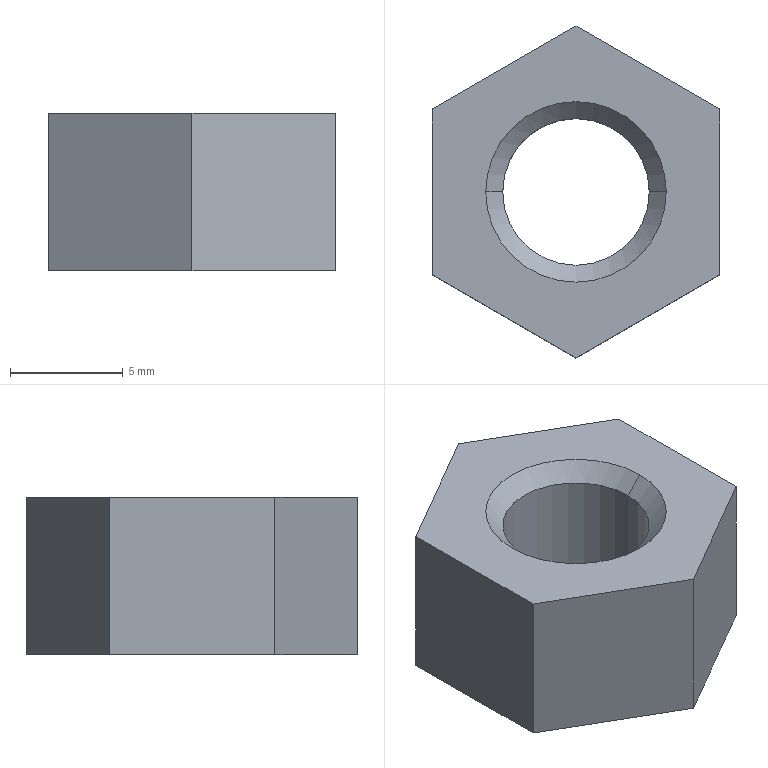Part | STEP file | Tan M8 | 1 solid | 14 faces | box 12.73 x 14.699 x 7 mm | volume 737.742 mm3 | plane 8 | cone 4 | cylinder 2 | commonest cylinder face diameters 6.5 x2
STEP:
#1=CARTESIAN_POINT('',(0.,0.,0.));
#2=DIRECTION('',(0.,0.,1.));
#3=DIRECTION('',(1.,0.,0.));
#4=AXIS2_PLACEMENT_3D('',#1,#2,#3);
#5=CARTESIAN_POINT('',(3.25,0.,6.25));
#6=VERTEX_POINT('',#5);
#7=CARTESIAN_POINT('',(4.,0.,7.));
#8=VERTEX_POINT('',#7);
#9=CARTESIAN_POINT('',(3.25,0.,6.25));
#10=DIRECTION('',(0.7071,0.,0.7071));
#11=VECTOR('',#10,1.);
#12=LINE('',#9,#11);
#13=CARTESIAN_POINT('',(0.,0.,6.25));
#14=DIRECTION('',(0.,0.,1.));
#15=DIRECTION('',(1.,0.,0.));
#16=AXIS2_PLACEMENT_3D('',#13,#14,#15);
#17=CONICAL_SURFACE('',#16,3.25,0.7854);
#18=CARTESIAN_POINT('',(6.283,0.));
#19=DIRECTION('',(0.,1.));
#20=VECTOR('',#19,1.);
#21=LINE('',#18,#20);
#22=(GEOMETRIC_REPRESENTATION_CONTEXT(2)PARAMETRIC_REPRESENTATION_CONTEXT()REPRESENTATION_CONTEXT('',''));
#23=DEFINITIONAL_REPRESENTATION('',(#21),#22);
#24=PCURVE('',#17,#23);
#25=CARTESIAN_POINT('',(0.,0.,6.25));
#26=DIRECTION('',(0.,0.,1.));
#27=DIRECTION('',(1.,0.,0.));
#28=AXIS2_PLACEMENT_3D('',#25,#26,#27);
#29=CONICAL_SURFACE('',#28,3.25,0.7854);
#30=CARTESIAN_POINT('',(0.,0.));
#31=DIRECTION('',(0.,1.));
#32=VECTOR('',#31,1.);
#33=LINE('',#30,#32);
#34=(GEOMETRIC_REPRESENTATION_CONTEXT(2)PARAMETRIC_REPRESENTATION_CONTEXT()REPRESENTATION_CONTEXT('',''));
#35=DEFINITIONAL_REPRESENTATION('',(#33),#34);
#36=PCURVE('',#29,#35);
#37=SURFACE_CURVE('',#12,(#24,#36),.PCURVE_S1.);
#38=EDGE_CURVE('',#6,#8,#37,.T.);
#39=ORIENTED_EDGE('',*,*,#38,.T.);
#40=CARTESIAN_POINT('',(-4.,0.,7.));
#41=VERTEX_POINT('',#40);
#42=CARTESIAN_POINT('',(0.,0.,7.));
#43=DIRECTION('',(0.,0.,-1.));
#44=DIRECTION('',(1.,0.,0.));
#45=AXIS2_PLACEMENT_3D('',#42,#43,#44);
#46=CIRCLE('',#45,4.);
#47=CARTESIAN_POINT('',(6.283,0.75));
#48=DIRECTION('',(-1.,0.));
#49=VECTOR('',#48,1.);
#50=LINE('',#47,#49);
#51=(GEOMETRIC_REPRESENTATION_CONTEXT(2)PARAMETRIC_REPRESENTATION_CONTEXT()REPRESENTATION_CONTEXT('',''));
#52=DEFINITIONAL_REPRESENTATION('',(#50),#51);
#53=PCURVE('',#17,#52);
#54=CARTESIAN_POINT('',(0.,0.,7.));
#55=DIRECTION('',(0.,0.,1.));
#56=DIRECTION('',(1.,0.,0.));
#57=AXIS2_PLACEMENT_3D('',#54,#55,#56);
#58=PLANE('',#57);
#59=CARTESIAN_POINT('',(4.,0.));
#60=CARTESIAN_POINT('',(4.,-6.928));
#61=CARTESIAN_POINT('',(-2.,-3.464));
#62=CARTESIAN_POINT('',(-8.,0.));
#63=CARTESIAN_POINT('',(-2.,3.464));
#64=CARTESIAN_POINT('',(4.,6.928));
#65=CARTESIAN_POINT('',(4.,0.));
#66=(BOUNDED_CURVE()B_SPLINE_CURVE(2,(#59,#60,#61,#62,#63,#64,#65),.UNSPECIFIED.,.T.,.F.)B_SPLINE_CURVE_WITH_KNOTS((1,2,2,2,2,1),(-2.094,0.,2.094,4.189,6.283,8.378),.UNSPECIFIED.)CURVE()GEOMETRIC_REPRESENTATION_ITEM()RATIONAL_B_SPLINE_CURVE((1.,0.5,1.,0.5,1.,0.5,1.))REPRESENTATION_ITEM(''));
#67=(GEOMETRIC_REPRESENTATION_CONTEXT(2)PARAMETRIC_REPRESENTATION_CONTEXT()REPRESENTATION_CONTEXT('',''));
#68=DEFINITIONAL_REPRESENTATION('',(#66),#67);
#69=PCURVE('',#58,#68);
#70=SURFACE_CURVE('',#46,(#53,#69),.PCURVE_S1.);
#71=EDGE_CURVE('',#8,#41,#70,.T.);
#72=ORIENTED_EDGE('',*,*,#71,.T.);
#73=CARTESIAN_POINT('',(-3.25,0.,6.25));
#74=VERTEX_POINT('',#73);
#75=CARTESIAN_POINT('',(-3.25,0.,6.25));
#76=DIRECTION('',(-0.7071,0.,0.7071));
#77=VECTOR('',#76,1.);
#78=LINE('',#75,#77);
#79=CARTESIAN_POINT('',(3.142,0.));
#80=DIRECTION('',(0.,1.));
#81=VECTOR('',#80,1.);
#82=LINE('',#79,#81);
#83=(GEOMETRIC_REPRESENTATION_CONTEXT(2)PARAMETRIC_REPRESENTATION_CONTEXT()REPRESENTATION_CONTEXT('',''));
#84=DEFINITIONAL_REPRESENTATION('',(#82),#83);
#85=PCURVE('',#17,#84);
#86=CARTESIAN_POINT('',(3.142,0.));
#87=DIRECTION('',(0.,1.));
#88=VECTOR('',#87,1.);
#89=LINE('',#86,#88);
#90=(GEOMETRIC_REPRESENTATION_CONTEXT(2)PARAMETRIC_REPRESENTATION_CONTEXT()REPRESENTATION_CONTEXT('',''));
#91=DEFINITIONAL_REPRESENTATION('',(#89),#90);
#92=PCURVE('',#29,#91);
#93=SURFACE_CURVE('',#78,(#85,#92),.PCURVE_S1.);
#94=EDGE_CURVE('',#74,#41,#93,.T.);
#95=ORIENTED_EDGE('',*,*,#94,.F.);
#96=CARTESIAN_POINT('',(0.,0.,6.25));
#97=DIRECTION('',(0.,0.,1.));
#98=DIRECTION('',(1.,0.,0.));
#99=AXIS2_PLACEMENT_3D('',#96,#97,#98);
#100=CIRCLE('',#99,3.25);
#101=CARTESIAN_POINT('',(0.,0.));
#102=DIRECTION('',(1.,0.));
#103=VECTOR('',#102,1.);
#104=LINE('',#101,#103);
#105=(GEOMETRIC_REPRESENTATION_CONTEXT(2)PARAMETRIC_REPRESENTATION_CONTEXT()REPRESENTATION_CONTEXT('',''));
#106=DEFINITIONAL_REPRESENTATION('',(#104),#105);
#107=PCURVE('',#17,#106);
#108=CARTESIAN_POINT('',(0.,0.,10.));
#109=DIRECTION('',(0.,0.,-1.));
#110=DIRECTION('',(-1.,0.,0.));
#111=AXIS2_PLACEMENT_3D('',#108,#109,#110);
#112=CYLINDRICAL_SURFACE('',#111,3.25);
#113=CARTESIAN_POINT('',(9.425,3.75));
#114=DIRECTION('',(-1.,0.));
#115=VECTOR('',#114,1.);
#116=LINE('',#113,#115);
#117=(GEOMETRIC_REPRESENTATION_CONTEXT(2)PARAMETRIC_REPRESENTATION_CONTEXT()REPRESENTATION_CONTEXT('',''));
#118=DEFINITIONAL_REPRESENTATION('',(#116),#117);
#119=PCURVE('',#112,#118);
#120=SURFACE_CURVE('',#100,(#107,#119),.PCURVE_S1.);
#121=EDGE_CURVE('',#74,#6,#120,.T.);
#122=ORIENTED_EDGE('',*,*,#121,.T.);
#123=EDGE_LOOP('',(#39,#72,#95,#122));
#124=FACE_BOUND('',#123,.F.);
#125=ADVANCED_FACE('',(#124),#17,.F.);
#126=CARTESIAN_POINT('',(-3.25,0.,0.75));
#127=VERTEX_POINT('',#126);
#128=CARTESIAN_POINT('',(-4.,0.,0.));
#129=VERTEX_POINT('',#128);
#130=CARTESIAN_POINT('',(-3.25,0.,0.75));
#131=DIRECTION('',(-0.7071,0.,-0.7071));
#132=VECTOR('',#131,1.);
#133=LINE('',#130,#132);
#134=CARTESIAN_POINT('',(0.,0.,0.75));
#135=DIRECTION('',(0.,0.,-1.));
#136=DIRECTION('',(-1.,0.,0.));
#137=AXIS2_PLACEMENT_3D('',#134,#135,#136);
#138=CONICAL_SURFACE('',#137,3.25,0.7854);
#139=CARTESIAN_POINT('',(6.283,0.));
#140=DIRECTION('',(0.,1.));
#141=VECTOR('',#140,1.);
#142=LINE('',#139,#141);
#143=(GEOMETRIC_REPRESENTATION_CONTEXT(2)PARAMETRIC_REPRESENTATION_CONTEXT()REPRESENTATION_CONTEXT('',''));
#144=DEFINITIONAL_REPRESENTATION('',(#142),#143);
#145=PCURVE('',#138,#144);
#146=CARTESIAN_POINT('',(0.,0.,0.75));
#147=DIRECTION('',(0.,0.,-1.));
#148=DIRECTION('',(-1.,0.,0.));
#149=AXIS2_PLACEMENT_3D('',#146,#147,#148);
#150=CONICAL_SURFACE('',#149,3.25,0.7854);
#151=CARTESIAN_POINT('',(0.,0.));
#152=DIRECTION('',(0.,1.));
#153=VECTOR('',#152,1.);
#154=LINE('',#151,#153);
#155=(GEOMETRIC_REPRESENTATION_CONTEXT(2)PARAMETRIC_REPRESENTATION_CONTEXT()REPRESENTATION_CONTEXT('',''));
#156=DEFINITIONAL_REPRESENTATION('',(#154),#155);
#157=PCURVE('',#150,#156);
#158=SURFACE_CURVE('',#133,(#145,#157),.PCURVE_S1.);
#159=EDGE_CURVE('',#127,#129,#158,.T.);
#160=ORIENTED_EDGE('',*,*,#159,.T.);
#161=CARTESIAN_POINT('',(4.,0.,0.));
#162=VERTEX_POINT('',#161);
#163=CARTESIAN_POINT('',(0.,0.,0.));
#164=DIRECTION('',(0.,0.,1.));
#165=DIRECTION('',(1.,0.,0.));
#166=AXIS2_PLACEMENT_3D('',#163,#164,#165);
#167=CIRCLE('',#166,4.);
#168=CARTESIAN_POINT('',(9.425,0.75));
#169=DIRECTION('',(-1.,0.));
#170=VECTOR('',#169,1.);
#171=LINE('',#168,#170);
#172=(GEOMETRIC_REPRESENTATION_CONTEXT(2)PARAMETRIC_REPRESENTATION_CONTEXT()REPRESENTATION_CONTEXT('',''));
#173=DEFINITIONAL_REPRESENTATION('',(#171),#172);
#174=PCURVE('',#138,#173);
#175=CARTESIAN_POINT('',(0.,0.,0.));
#176=DIRECTION('',(0.,0.,1.));
#177=DIRECTION('',(1.,0.,0.));
#178=AXIS2_PLACEMENT_3D('',#175,#176,#177);
#179=PLANE('',#178);
#180=CARTESIAN_POINT('',(0.,0.));
#181=DIRECTION('',(1.,0.));
#182=AXIS2_PLACEMENT_2D('',#180,#181);
#183=CIRCLE('',#182,4.);
#184=(GEOMETRIC_REPRESENTATION_CONTEXT(2)PARAMETRIC_REPRESENTATION_CONTEXT()REPRESENTATION_CONTEXT('',''));
#185=DEFINITIONAL_REPRESENTATION('',(#183),#184);
#186=PCURVE('',#179,#185);
#187=SURFACE_CURVE('',#167,(#174,#186),.PCURVE_S1.);
#188=EDGE_CURVE('',#129,#162,#187,.T.);
#189=ORIENTED_EDGE('',*,*,#188,.T.);
#190=CARTESIAN_POINT('',(3.25,0.,0.75));
#191=VERTEX_POINT('',#190);
#192=CARTESIAN_POINT('',(3.25,0.,0.75));
#193=DIRECTION('',(0.7071,0.,-0.7071));
#194=VECTOR('',#193,1.);
#195=LINE('',#192,#194);
#196=CARTESIAN_POINT('',(3.142,0.));
#197=DIRECTION('',(0.,1.));
#198=VECTOR('',#197,1.);
#199=LINE('',#196,#198);
#200=(GEOMETRIC_REPRESENTATION_CONTEXT(2)PARAMETRIC_REPRESENTATION_CONTEXT()REPRESENTATION_CONTEXT('',''));
#201=DEFINITIONAL_REPRESENTATION('',(#199),#200);
#202=PCURVE('',#138,#201);
#203=CARTESIAN_POINT('',(3.142,0.));
#204=DIRECTION('',(0.,1.));
#205=VECTOR('',#204,1.);
#206=LINE('',#203,#205);
#207=(GEOMETRIC_REPRESENTATION_CONTEXT(2)PARAMETRIC_REPRESENTATION_CONTEXT()REPRESENTATION_CONTEXT('',''));
#208=DEFINITIONAL_REPRESENTATION('',(#206),#207);
#209=PCURVE('',#150,#208);
#210=SURFACE_CURVE('',#195,(#202,#209),.PCURVE_S1.);
#211=EDGE_CURVE('',#191,#162,#210,.T.);
#212=ORIENTED_EDGE('',*,*,#211,.F.);
#213=CARTESIAN_POINT('',(0.,0.,0.75));
#214=DIRECTION('',(0.,0.,-1.));
#215=DIRECTION('',(1.,0.,0.));
#216=AXIS2_PLACEMENT_3D('',#213,#214,#215);
#217=CIRCLE('',#216,3.25);
#218=CARTESIAN_POINT('',(3.142,0.));
#219=DIRECTION('',(1.,0.));
#220=VECTOR('',#219,1.);
#221=LINE('',#218,#220);
#222=(GEOMETRIC_REPRESENTATION_CONTEXT(2)PARAMETRIC_REPRESENTATION_CONTEXT()REPRESENTATION_CONTEXT('',''));
#223=DEFINITIONAL_REPRESENTATION('',(#221),#222);
#224=PCURVE('',#138,#223);
#225=CARTESIAN_POINT('',(3.142,9.25));
#226=DIRECTION('',(1.,0.));
#227=VECTOR('',#226,1.);
#228=LINE('',#225,#227);
#229=(GEOMETRIC_REPRESENTATION_CONTEXT(2)PARAMETRIC_REPRESENTATION_CONTEXT()REPRESENTATION_CONTEXT('',''));
#230=DEFINITIONAL_REPRESENTATION('',(#228),#229);
#231=PCURVE('',#112,#230);
#232=SURFACE_CURVE('',#217,(#224,#231),.PCURVE_S1.);
#233=EDGE_CURVE('',#191,#127,#232,.T.);
#234=ORIENTED_EDGE('',*,*,#233,.T.);
#235=EDGE_LOOP('',(#160,#189,#212,#234));
#236=FACE_BOUND('',#235,.F.);
#237=ADVANCED_FACE('',(#236),#138,.F.);
#238=CARTESIAN_POINT('',(-3.25,0.,10.));
#239=DIRECTION('',(0.,0.,-1.));
#240=VECTOR('',#239,1.);
#241=LINE('',#238,#240);
#242=CARTESIAN_POINT('',(6.283,0.));
#243=DIRECTION('',(0.,1.));
#244=VECTOR('',#243,1.);
#245=LINE('',#242,#244);
#246=(GEOMETRIC_REPRESENTATION_CONTEXT(2)PARAMETRIC_REPRESENTATION_CONTEXT()REPRESENTATION_CONTEXT('',''));
#247=DEFINITIONAL_REPRESENTATION('',(#245),#246);
#248=PCURVE('',#112,#247);
#249=CARTESIAN_POINT('',(0.,0.,10.));
#250=DIRECTION('',(0.,0.,-1.));
#251=DIRECTION('',(-1.,0.,0.));
#252=AXIS2_PLACEMENT_3D('',#249,#250,#251);
#253=CYLINDRICAL_SURFACE('',#252,3.25);
#254=CARTESIAN_POINT('',(0.,0.));
#255=DIRECTION('',(0.,1.));
#256=VECTOR('',#255,1.);
#257=LINE('',#254,#256);
#258=(GEOMETRIC_REPRESENTATION_CONTEXT(2)PARAMETRIC_REPRESENTATION_CONTEXT()REPRESENTATION_CONTEXT('',''));
#259=DEFINITIONAL_REPRESENTATION('',(#257),#258);
#260=PCURVE('',#253,#259);
#261=SURFACE_CURVE('',#241,(#248,#260),.PCURVE_S1.);
#262=EDGE_CURVE('',#74,#127,#261,.T.);
#263=ORIENTED_EDGE('',*,*,#262,.T.);
#264=ORIENTED_EDGE('',*,*,#233,.F.);
#265=CARTESIAN_POINT('',(3.25,0.,10.));
#266=DIRECTION('',(0.,0.,-1.));
#267=VECTOR('',#266,1.);
#268=LINE('',#265,#267);
#269=CARTESIAN_POINT('',(3.142,0.));
#270=DIRECTION('',(0.,1.));
#271=VECTOR('',#270,1.);
#272=LINE('',#269,#271);
#273=(GEOMETRIC_REPRESENTATION_CONTEXT(2)PARAMETRIC_REPRESENTATION_CONTEXT()REPRESENTATION_CONTEXT('',''));
#274=DEFINITIONAL_REPRESENTATION('',(#272),#273);
#275=PCURVE('',#112,#274);
#276=CARTESIAN_POINT('',(3.142,0.));
#277=DIRECTION('',(0.,1.));
#278=VECTOR('',#277,1.);
#279=LINE('',#276,#278);
#280=(GEOMETRIC_REPRESENTATION_CONTEXT(2)PARAMETRIC_REPRESENTATION_CONTEXT()REPRESENTATION_CONTEXT('',''));
#281=DEFINITIONAL_REPRESENTATION('',(#279),#280);
#282=PCURVE('',#253,#281);
#283=SURFACE_CURVE('',#268,(#275,#282),.PCURVE_S1.);
#284=EDGE_CURVE('',#6,#191,#283,.T.);
#285=ORIENTED_EDGE('',*,*,#284,.F.);
#286=ORIENTED_EDGE('',*,*,#121,.F.);
#287=EDGE_LOOP('',(#263,#264,#285,#286));
#288=FACE_BOUND('',#287,.F.);
#289=ADVANCED_FACE('',(#288),#112,.F.);
#290=CARTESIAN_POINT('',(6.365,3.675,0.));
#291=VERTEX_POINT('',#290);
#292=CARTESIAN_POINT('',(0.,7.35,0.));
#293=VERTEX_POINT('',#292);
#294=CARTESIAN_POINT('',(6.365,3.675,0.));
#295=DIRECTION('',(-0.866,0.5,0.));
#296=VECTOR('',#295,1.);
#297=LINE('',#294,#296);
#298=CARTESIAN_POINT('',(6.365,3.675,7.));
#299=DIRECTION('',(-0.5,-0.866,0.));
#300=DIRECTION('',(0.866,-0.5,0.));
#301=AXIS2_PLACEMENT_3D('',#298,#299,#300);
#302=PLANE('',#301);
#303=CARTESIAN_POINT('',(0.,-7.));
#304=DIRECTION('',(-1.,0.));
#305=VECTOR('',#304,1.);
#306=LINE('',#303,#305);
#307=(GEOMETRIC_REPRESENTATION_CONTEXT(2)PARAMETRIC_REPRESENTATION_CONTEXT()REPRESENTATION_CONTEXT('',''));
#308=DEFINITIONAL_REPRESENTATION('',(#306),#307);
#309=PCURVE('',#302,#308);
#310=CARTESIAN_POINT('',(6.365,3.675));
#311=DIRECTION('',(-0.866,0.5));
#312=VECTOR('',#311,1.);
#313=LINE('',#310,#312);
#314=(GEOMETRIC_REPRESENTATION_CONTEXT(2)PARAMETRIC_REPRESENTATION_CONTEXT()REPRESENTATION_CONTEXT('',''));
#315=DEFINITIONAL_REPRESENTATION('',(#313),#314);
#316=PCURVE('',#179,#315);
#317=SURFACE_CURVE('',#297,(#309,#316),.PCURVE_S1.);
#318=EDGE_CURVE('',#291,#293,#317,.T.);
#319=ORIENTED_EDGE('',*,*,#318,.T.);
#320=CARTESIAN_POINT('',(0.,7.35,7.));
#321=VERTEX_POINT('',#320);
#322=CARTESIAN_POINT('',(0.,7.35,7.));
#323=DIRECTION('',(0.,0.,-1.));
#324=VECTOR('',#323,1.);
#325=LINE('',#322,#324);
#326=CARTESIAN_POINT('',(-7.35,0.));
#327=DIRECTION('',(0.,-1.));
#328=VECTOR('',#327,1.);
#329=LINE('',#326,#328);
#330=(GEOMETRIC_REPRESENTATION_CONTEXT(2)PARAMETRIC_REPRESENTATION_CONTEXT()REPRESENTATION_CONTEXT('',''));
#331=DEFINITIONAL_REPRESENTATION('',(#329),#330);
#332=PCURVE('',#302,#331);
#333=CARTESIAN_POINT('',(0.,7.35,7.));
#334=DIRECTION('',(0.5,-0.866,0.));
#335=DIRECTION('',(0.866,0.5,0.));
#336=AXIS2_PLACEMENT_3D('',#333,#334,#335);
#337=PLANE('',#336);
#338=CARTESIAN_POINT('',(0.,0.));
#339=DIRECTION('',(0.,-1.));
#340=VECTOR('',#339,1.);
#341=LINE('',#338,#340);
#342=(GEOMETRIC_REPRESENTATION_CONTEXT(2)PARAMETRIC_REPRESENTATION_CONTEXT()REPRESENTATION_CONTEXT('',''));
#343=DEFINITIONAL_REPRESENTATION('',(#341),#342);
#344=PCURVE('',#337,#343);
#345=SURFACE_CURVE('',#325,(#332,#344),.PCURVE_S1.);
#346=EDGE_CURVE('',#321,#293,#345,.T.);
#347=ORIENTED_EDGE('',*,*,#346,.F.);
#348=CARTESIAN_POINT('',(6.365,3.675,7.));
#349=VERTEX_POINT('',#348);
#350=CARTESIAN_POINT('',(6.365,3.675,7.));
#351=DIRECTION('',(-0.866,0.5,0.));
#352=VECTOR('',#351,1.);
#353=LINE('',#350,#352);
#354=CARTESIAN_POINT('',(0.,0.));
#355=DIRECTION('',(-1.,0.));
#356=VECTOR('',#355,1.);
#357=LINE('',#354,#356);
#358=(GEOMETRIC_REPRESENTATION_CONTEXT(2)PARAMETRIC_REPRESENTATION_CONTEXT()REPRESENTATION_CONTEXT('',''));
#359=DEFINITIONAL_REPRESENTATION('',(#357),#358);
#360=PCURVE('',#302,#359);
#361=CARTESIAN_POINT('',(6.365,3.675));
#362=DIRECTION('',(-0.866,0.5));
#363=VECTOR('',#362,1.);
#364=LINE('',#361,#363);
#365=(GEOMETRIC_REPRESENTATION_CONTEXT(2)PARAMETRIC_REPRESENTATION_CONTEXT()REPRESENTATION_CONTEXT('',''));
#366=DEFINITIONAL_REPRESENTATION('',(#364),#365);
#367=PCURVE('',#58,#366);
#368=SURFACE_CURVE('',#353,(#360,#367),.PCURVE_S1.);
#369=EDGE_CURVE('',#349,#321,#368,.T.);
#370=ORIENTED_EDGE('',*,*,#369,.F.);
#371=CARTESIAN_POINT('',(6.365,3.675,7.));
#372=DIRECTION('',(0.,0.,-1.));
#373=VECTOR('',#372,1.);
#374=LINE('',#371,#373);
#375=CARTESIAN_POINT('',(0.,0.));
#376=DIRECTION('',(0.,-1.));
#377=VECTOR('',#376,1.);
#378=LINE('',#375,#377);
#379=(GEOMETRIC_REPRESENTATION_CONTEXT(2)PARAMETRIC_REPRESENTATION_CONTEXT()REPRESENTATION_CONTEXT('',''));
#380=DEFINITIONAL_REPRESENTATION('',(#378),#379);
#381=PCURVE('',#302,#380);
#382=CARTESIAN_POINT('',(6.365,-3.675,7.));
#383=DIRECTION('',(-1.,0.,0.));
#384=DIRECTION('',(0.,-1.,0.));
#385=AXIS2_PLACEMENT_3D('',#382,#383,#384);
#386=PLANE('',#385);
#387=CARTESIAN_POINT('',(-7.35,0.));
#388=DIRECTION('',(0.,-1.));
#389=VECTOR('',#388,1.);
#390=LINE('',#387,#389);
#391=(GEOMETRIC_REPRESENTATION_CONTEXT(2)PARAMETRIC_REPRESENTATION_CONTEXT()REPRESENTATION_CONTEXT('',''));
#392=DEFINITIONAL_REPRESENTATION('',(#390),#391);
#393=PCURVE('',#386,#392);
#394=SURFACE_CURVE('',#374,(#381,#393),.PCURVE_S1.);
#395=EDGE_CURVE('',#349,#291,#394,.T.);
#396=ORIENTED_EDGE('',*,*,#395,.T.);
#397=EDGE_LOOP('',(#319,#347,#370,#396));
#398=FACE_BOUND('',#397,.T.);
#399=ADVANCED_FACE('',(#398),#302,.F.);
#400=CARTESIAN_POINT('',(-6.365,3.675,0.));
#401=VERTEX_POINT('',#400);
#402=CARTESIAN_POINT('',(0.,7.35,0.));
#403=DIRECTION('',(-0.866,-0.5,0.));
#404=VECTOR('',#403,1.);
#405=LINE('',#402,#404);
#406=CARTESIAN_POINT('',(0.,-7.));
#407=DIRECTION('',(-1.,0.));
#408=VECTOR('',#407,1.);
#409=LINE('',#406,#408);
#410=(GEOMETRIC_REPRESENTATION_CONTEXT(2)PARAMETRIC_REPRESENTATION_CONTEXT()REPRESENTATION_CONTEXT('',''));
#411=DEFINITIONAL_REPRESENTATION('',(#409),#410);
#412=PCURVE('',#337,#411);
#413=CARTESIAN_POINT('',(0.,7.35));
#414=DIRECTION('',(-0.866,-0.5));
#415=VECTOR('',#414,1.);
#416=LINE('',#413,#415);
#417=(GEOMETRIC_REPRESENTATION_CONTEXT(2)PARAMETRIC_REPRESENTATION_CONTEXT()REPRESENTATION_CONTEXT('',''));
#418=DEFINITIONAL_REPRESENTATION('',(#416),#417);
#419=PCURVE('',#179,#418);
#420=SURFACE_CURVE('',#405,(#412,#419),.PCURVE_S1.);
#421=EDGE_CURVE('',#293,#401,#420,.T.);
#422=ORIENTED_EDGE('',*,*,#421,.T.);
#423=CARTESIAN_POINT('',(-6.365,3.675,7.));
#424=VERTEX_POINT('',#423);
#425=CARTESIAN_POINT('',(-6.365,3.675,7.));
#426=DIRECTION('',(0.,0.,-1.));
#427=VECTOR('',#426,1.);
#428=LINE('',#425,#427);
#429=CARTESIAN_POINT('',(-7.35,0.));
#430=DIRECTION('',(0.,-1.));
#431=VECTOR('',#430,1.);
#432=LINE('',#429,#431);
#433=(GEOMETRIC_REPRESENTATION_CONTEXT(2)PARAMETRIC_REPRESENTATION_CONTEXT()REPRESENTATION_CONTEXT('',''));
#434=DEFINITIONAL_REPRESENTATION('',(#432),#433);
#435=PCURVE('',#337,#434);
#436=CARTESIAN_POINT('',(-6.365,3.675,7.));
#437=DIRECTION('',(1.,0.,0.));
#438=DIRECTION('',(0.,0.,-1.));
#439=AXIS2_PLACEMENT_3D('',#436,#437,#438);
#440=PLANE('',#439);
#441=CARTESIAN_POINT('',(0.,0.));
#442=DIRECTION('',(1.,0.));
#443=VECTOR('',#442,1.);
#444=LINE('',#441,#443);
#445=(GEOMETRIC_REPRESENTATION_CONTEXT(2)PARAMETRIC_REPRESENTATION_CONTEXT()REPRESENTATION_CONTEXT('',''));
#446=DEFINITIONAL_REPRESENTATION('',(#444),#445);
#447=PCURVE('',#440,#446);
#448=SURFACE_CURVE('',#428,(#435,#447),.PCURVE_S1.);
#449=EDGE_CURVE('',#424,#401,#448,.T.);
#450=ORIENTED_EDGE('',*,*,#449,.F.);
#451=CARTESIAN_POINT('',(0.,7.35,7.));
#452=DIRECTION('',(-0.866,-0.5,0.));
#453=VECTOR('',#452,1.);
#454=LINE('',#451,#453);
#455=CARTESIAN_POINT('',(0.,0.));
#456=DIRECTION('',(-1.,0.));
#457=VECTOR('',#456,1.);
#458=LINE('',#455,#457);
#459=(GEOMETRIC_REPRESENTATION_CONTEXT(2)PARAMETRIC_REPRESENTATION_CONTEXT()REPRESENTATION_CONTEXT('',''));
#460=DEFINITIONAL_REPRESENTATION('',(#458),#459);
#461=PCURVE('',#337,#460);
#462=CARTESIAN_POINT('',(0.,7.35));
#463=DIRECTION('',(-0.866,-0.5));
#464=VECTOR('',#463,1.);
#465=LINE('',#462,#464);
#466=(GEOMETRIC_REPRESENTATION_CONTEXT(2)PARAMETRIC_REPRESENTATION_CONTEXT()REPRESENTATION_CONTEXT('',''));
#467=DEFINITIONAL_REPRESENTATION('',(#465),#466);
#468=PCURVE('',#58,#467);
#469=SURFACE_CURVE('',#454,(#461,#468),.PCURVE_S1.);
#470=EDGE_CURVE('',#321,#424,#469,.T.);
#471=ORIENTED_EDGE('',*,*,#470,.F.);
#472=ORIENTED_EDGE('',*,*,#346,.T.);
#473=EDGE_LOOP('',(#422,#450,#471,#472));
#474=FACE_BOUND('',#473,.T.);
#475=ADVANCED_FACE('',(#474),#337,.F.);
#476=CARTESIAN_POINT('',(-6.365,-3.675,0.));
#477=VERTEX_POINT('',#476);
#478=CARTESIAN_POINT('',(-6.365,3.675,0.));
#479=DIRECTION('',(0.,-1.,0.));
#480=VECTOR('',#479,1.);
#481=LINE('',#478,#480);
#482=CARTESIAN_POINT('',(7.,0.));
#483=DIRECTION('',(0.,-1.));
#484=VECTOR('',#483,1.);
#485=LINE('',#482,#484);
#486=(GEOMETRIC_REPRESENTATION_CONTEXT(2)PARAMETRIC_REPRESENTATION_CONTEXT()REPRESENTATION_CONTEXT('',''));
#487=DEFINITIONAL_REPRESENTATION('',(#485),#486);
#488=PCURVE('',#440,#487);
#489=CARTESIAN_POINT('',(-6.365,3.675));
#490=DIRECTION('',(0.,-1.));
#491=VECTOR('',#490,1.);
#492=LINE('',#489,#491);
#493=(GEOMETRIC_REPRESENTATION_CONTEXT(2)PARAMETRIC_REPRESENTATION_CONTEXT()REPRESENTATION_CONTEXT('',''));
#494=DEFINITIONAL_REPRESENTATION('',(#492),#493);
#495=PCURVE('',#179,#494);
#496=SURFACE_CURVE('',#481,(#488,#495),.PCURVE_S1.);
#497=EDGE_CURVE('',#401,#477,#496,.T.);
#498=ORIENTED_EDGE('',*,*,#497,.T.);
#499=CARTESIAN_POINT('',(-6.365,-3.675,7.));
#500=VERTEX_POINT('',#499);
#501=CARTESIAN_POINT('',(-6.365,-3.675,7.));
#502=DIRECTION('',(0.,0.,-1.));
#503=VECTOR('',#502,1.);
#504=LINE('',#501,#503);
#505=CARTESIAN_POINT('',(0.,-7.35));
#506=DIRECTION('',(1.,0.));
#507=VECTOR('',#506,1.);
#508=LINE('',#505,#507);
#509=(GEOMETRIC_REPRESENTATION_CONTEXT(2)PARAMETRIC_REPRESENTATION_CONTEXT()REPRESENTATION_CONTEXT('',''));
#510=DEFINITIONAL_REPRESENTATION('',(#508),#509);
#511=PCURVE('',#440,#510);
#512=CARTESIAN_POINT('',(-6.365,-3.675,7.));
#513=DIRECTION('',(0.5,0.866,0.));
#514=DIRECTION('',(-0.866,0.5,0.));
#515=AXIS2_PLACEMENT_3D('',#512,#513,#514);
#516=PLANE('',#515);
#517=CARTESIAN_POINT('',(0.,0.));
#518=DIRECTION('',(0.,-1.));
#519=VECTOR('',#518,1.);
#520=LINE('',#517,#519);
#521=(GEOMETRIC_REPRESENTATION_CONTEXT(2)PARAMETRIC_REPRESENTATION_CONTEXT()REPRESENTATION_CONTEXT('',''));
#522=DEFINITIONAL_REPRESENTATION('',(#520),#521);
#523=PCURVE('',#516,#522);
#524=SURFACE_CURVE('',#504,(#511,#523),.PCURVE_S1.);
#525=EDGE_CURVE('',#500,#477,#524,.T.);
#526=ORIENTED_EDGE('',*,*,#525,.F.);
#527=CARTESIAN_POINT('',(-6.365,3.675,7.));
#528=DIRECTION('',(0.,-1.,0.));
#529=VECTOR('',#528,1.);
#530=LINE('',#527,#529);
#531=CARTESIAN_POINT('',(0.,0.));
#532=DIRECTION('',(0.,-1.));
#533=VECTOR('',#532,1.);
#534=LINE('',#531,#533);
#535=(GEOMETRIC_REPRESENTATION_CONTEXT(2)PARAMETRIC_REPRESENTATION_CONTEXT()REPRESENTATION_CONTEXT('',''));
#536=DEFINITIONAL_REPRESENTATION('',(#534),#535);
#537=PCURVE('',#440,#536);
#538=CARTESIAN_POINT('',(-6.365,3.675));
#539=DIRECTION('',(0.,-1.));
#540=VECTOR('',#539,1.);
#541=LINE('',#538,#540);
#542=(GEOMETRIC_REPRESENTATION_CONTEXT(2)PARAMETRIC_REPRESENTATION_CONTEXT()REPRESENTATION_CONTEXT('',''));
#543=DEFINITIONAL_REPRESENTATION('',(#541),#542);
#544=PCURVE('',#58,#543);
#545=SURFACE_CURVE('',#530,(#537,#544),.PCURVE_S1.);
#546=EDGE_CURVE('',#424,#500,#545,.T.);
#547=ORIENTED_EDGE('',*,*,#546,.F.);
#548=ORIENTED_EDGE('',*,*,#449,.T.);
#549=EDGE_LOOP('',(#498,#526,#547,#548));
#550=FACE_BOUND('',#549,.T.);
#551=ADVANCED_FACE('',(#550),#440,.F.);
#552=CARTESIAN_POINT('',(0.,-7.35,0.));
#553=VERTEX_POINT('',#552);
#554=CARTESIAN_POINT('',(-6.365,-3.675,0.));
#555=DIRECTION('',(0.866,-0.5,0.));
#556=VECTOR('',#555,1.);
#557=LINE('',#554,#556);
#558=CARTESIAN_POINT('',(0.,-7.));
#559=DIRECTION('',(-1.,0.));
#560=VECTOR('',#559,1.);
#561=LINE('',#558,#560);
#562=(GEOMETRIC_REPRESENTATION_CONTEXT(2)PARAMETRIC_REPRESENTATION_CONTEXT()REPRESENTATION_CONTEXT('',''));
#563=DEFINITIONAL_REPRESENTATION('',(#561),#562);
#564=PCURVE('',#516,#563);
#565=CARTESIAN_POINT('',(-6.365,-3.675));
#566=DIRECTION('',(0.866,-0.5));
#567=VECTOR('',#566,1.);
#568=LINE('',#565,#567);
#569=(GEOMETRIC_REPRESENTATION_CONTEXT(2)PARAMETRIC_REPRESENTATION_CONTEXT()REPRESENTATION_CONTEXT('',''));
#570=DEFINITIONAL_REPRESENTATION('',(#568),#569);
#571=PCURVE('',#179,#570);
#572=SURFACE_CURVE('',#557,(#564,#571),.PCURVE_S1.);
#573=EDGE_CURVE('',#477,#553,#572,.T.);
#574=ORIENTED_EDGE('',*,*,#573,.T.);
#575=CARTESIAN_POINT('',(0.,-7.35,7.));
#576=VERTEX_POINT('',#575);
#577=CARTESIAN_POINT('',(0.,-7.35,7.));
#578=DIRECTION('',(0.,0.,-1.));
#579=VECTOR('',#578,1.);
#580=LINE('',#577,#579);
#581=CARTESIAN_POINT('',(-7.35,0.));
#582=DIRECTION('',(0.,-1.));
#583=VECTOR('',#582,1.);
#584=LINE('',#581,#583);
#585=(GEOMETRIC_REPRESENTATION_CONTEXT(2)PARAMETRIC_REPRESENTATION_CONTEXT()REPRESENTATION_CONTEXT('',''));
#586=DEFINITIONAL_REPRESENTATION('',(#584),#585);
#587=PCURVE('',#516,#586);
#588=CARTESIAN_POINT('',(0.,-7.35,7.));
#589=DIRECTION('',(-0.5,0.866,0.));
#590=DIRECTION('',(-0.866,-0.5,0.));
#591=AXIS2_PLACEMENT_3D('',#588,#589,#590);
#592=PLANE('',#591);
#593=CARTESIAN_POINT('',(0.,0.));
#594=DIRECTION('',(0.,-1.));
#595=VECTOR('',#594,1.);
#596=LINE('',#593,#595);
#597=(GEOMETRIC_REPRESENTATION_CONTEXT(2)PARAMETRIC_REPRESENTATION_CONTEXT()REPRESENTATION_CONTEXT('',''));
#598=DEFINITIONAL_REPRESENTATION('',(#596),#597);
#599=PCURVE('',#592,#598);
#600=SURFACE_CURVE('',#580,(#587,#599),.PCURVE_S1.);
#601=EDGE_CURVE('',#576,#553,#600,.T.);
#602=ORIENTED_EDGE('',*,*,#601,.F.);
#603=CARTESIAN_POINT('',(-6.365,-3.675,7.));
#604=DIRECTION('',(0.866,-0.5,0.));
#605=VECTOR('',#604,1.);
#606=LINE('',#603,#605);
#607=CARTESIAN_POINT('',(0.,0.));
#608=DIRECTION('',(-1.,0.));
#609=VECTOR('',#608,1.);
#610=LINE('',#607,#609);
#611=(GEOMETRIC_REPRESENTATION_CONTEXT(2)PARAMETRIC_REPRESENTATION_CONTEXT()REPRESENTATION_CONTEXT('',''));
#612=DEFINITIONAL_REPRESENTATION('',(#610),#611);
#613=PCURVE('',#516,#612);
#614=CARTESIAN_POINT('',(-6.365,-3.675));
#615=DIRECTION('',(0.866,-0.5));
#616=VECTOR('',#615,1.);
#617=LINE('',#614,#616);
#618=(GEOMETRIC_REPRESENTATION_CONTEXT(2)PARAMETRIC_REPRESENTATION_CONTEXT()REPRESENTATION_CONTEXT('',''));
#619=DEFINITIONAL_REPRESENTATION('',(#617),#618);
#620=PCURVE('',#58,#619);
#621=SURFACE_CURVE('',#606,(#613,#620),.PCURVE_S1.);
#622=EDGE_CURVE('',#500,#576,#621,.T.);
#623=ORIENTED_EDGE('',*,*,#622,.F.);
#624=ORIENTED_EDGE('',*,*,#525,.T.);
#625=EDGE_LOOP('',(#574,#602,#623,#624));
#626=FACE_BOUND('',#625,.T.);
#627=ADVANCED_FACE('',(#626),#516,.F.);
#628=CARTESIAN_POINT('',(6.365,-3.675,0.));
#629=VERTEX_POINT('',#628);
#630=CARTESIAN_POINT('',(0.,-7.35,0.));
#631=DIRECTION('',(0.866,0.5,0.));
#632=VECTOR('',#631,1.);
#633=LINE('',#630,#632);
#634=CARTESIAN_POINT('',(0.,-7.));
#635=DIRECTION('',(-1.,0.));
#636=VECTOR('',#635,1.);
#637=LINE('',#634,#636);
#638=(GEOMETRIC_REPRESENTATION_CONTEXT(2)PARAMETRIC_REPRESENTATION_CONTEXT()REPRESENTATION_CONTEXT('',''));
#639=DEFINITIONAL_REPRESENTATION('',(#637),#638);
#640=PCURVE('',#592,#639);
#641=CARTESIAN_POINT('',(0.,-7.35));
#642=DIRECTION('',(0.866,0.5));
#643=VECTOR('',#642,1.);
#644=LINE('',#641,#643);
#645=(GEOMETRIC_REPRESENTATION_CONTEXT(2)PARAMETRIC_REPRESENTATION_CONTEXT()REPRESENTATION_CONTEXT('',''));
#646=DEFINITIONAL_REPRESENTATION('',(#644),#645);
#647=PCURVE('',#179,#646);
#648=SURFACE_CURVE('',#633,(#640,#647),.PCURVE_S1.);
#649=EDGE_CURVE('',#553,#629,#648,.T.);
#650=ORIENTED_EDGE('',*,*,#649,.T.);
#651=CARTESIAN_POINT('',(6.365,-3.675,7.));
#652=VERTEX_POINT('',#651);
#653=CARTESIAN_POINT('',(6.365,-3.675,7.));
#654=DIRECTION('',(0.,0.,-1.));
#655=VECTOR('',#654,1.);
#656=LINE('',#653,#655);
#657=CARTESIAN_POINT('',(-7.35,0.));
#658=DIRECTION('',(0.,-1.));
#659=VECTOR('',#658,1.);
#660=LINE('',#657,#659);
#661=(GEOMETRIC_REPRESENTATION_CONTEXT(2)PARAMETRIC_REPRESENTATION_CONTEXT()REPRESENTATION_CONTEXT('',''));
#662=DEFINITIONAL_REPRESENTATION('',(#660),#661);
#663=PCURVE('',#592,#662);
#664=CARTESIAN_POINT('',(0.,0.));
#665=DIRECTION('',(0.,-1.));
#666=VECTOR('',#665,1.);
#667=LINE('',#664,#666);
#668=(GEOMETRIC_REPRESENTATION_CONTEXT(2)PARAMETRIC_REPRESENTATION_CONTEXT()REPRESENTATION_CONTEXT('',''));
#669=DEFINITIONAL_REPRESENTATION('',(#667),#668);
#670=PCURVE('',#386,#669);
#671=SURFACE_CURVE('',#656,(#663,#670),.PCURVE_S1.);
#672=EDGE_CURVE('',#652,#629,#671,.T.);
#673=ORIENTED_EDGE('',*,*,#672,.F.);
#674=CARTESIAN_POINT('',(0.,-7.35,7.));
#675=DIRECTION('',(0.866,0.5,0.));
#676=VECTOR('',#675,1.);
#677=LINE('',#674,#676);
#678=CARTESIAN_POINT('',(0.,0.));
#679=DIRECTION('',(-1.,0.));
#680=VECTOR('',#679,1.);
#681=LINE('',#678,#680);
#682=(GEOMETRIC_REPRESENTATION_CONTEXT(2)PARAMETRIC_REPRESENTATION_CONTEXT()REPRESENTATION_CONTEXT('',''));
#683=DEFINITIONAL_REPRESENTATION('',(#681),#682);
#684=PCURVE('',#592,#683);
#685=CARTESIAN_POINT('',(0.,-7.35));
#686=DIRECTION('',(0.866,0.5));
#687=VECTOR('',#686,1.);
#688=LINE('',#685,#687);
#689=(GEOMETRIC_REPRESENTATION_CONTEXT(2)PARAMETRIC_REPRESENTATION_CONTEXT()REPRESENTATION_CONTEXT('',''));
#690=DEFINITIONAL_REPRESENTATION('',(#688),#689);
#691=PCURVE('',#58,#690);
#692=SURFACE_CURVE('',#677,(#684,#691),.PCURVE_S1.);
#693=EDGE_CURVE('',#576,#652,#692,.T.);
#694=ORIENTED_EDGE('',*,*,#693,.F.);
#695=ORIENTED_EDGE('',*,*,#601,.T.);
#696=EDGE_LOOP('',(#650,#673,#694,#695));
#697=FACE_BOUND('',#696,.T.);
#698=ADVANCED_FACE('',(#697),#592,.F.);
#699=CARTESIAN_POINT('',(6.365,-3.675,0.));
#700=DIRECTION('',(0.,1.,0.));
#701=VECTOR('',#700,1.);
#702=LINE('',#699,#701);
#703=CARTESIAN_POINT('',(0.,-7.));
#704=DIRECTION('',(-1.,0.));
#705=VECTOR('',#704,1.);
#706=LINE('',#703,#705);
#707=(GEOMETRIC_REPRESENTATION_CONTEXT(2)PARAMETRIC_REPRESENTATION_CONTEXT()REPRESENTATION_CONTEXT('',''));
#708=DEFINITIONAL_REPRESENTATION('',(#706),#707);
#709=PCURVE('',#386,#708);
#710=CARTESIAN_POINT('',(6.365,-3.675));
#711=DIRECTION('',(0.,1.));
#712=VECTOR('',#711,1.);
#713=LINE('',#710,#712);
#714=(GEOMETRIC_REPRESENTATION_CONTEXT(2)PARAMETRIC_REPRESENTATION_CONTEXT()REPRESENTATION_CONTEXT('',''));
#715=DEFINITIONAL_REPRESENTATION('',(#713),#714);
#716=PCURVE('',#179,#715);
#717=SURFACE_CURVE('',#702,(#709,#716),.PCURVE_S1.);
#718=EDGE_CURVE('',#629,#291,#717,.T.);
#719=ORIENTED_EDGE('',*,*,#718,.T.);
#720=ORIENTED_EDGE('',*,*,#395,.F.);
#721=CARTESIAN_POINT('',(6.365,-3.675,7.));
#722=DIRECTION('',(0.,1.,0.));
#723=VECTOR('',#722,1.);
#724=LINE('',#721,#723);
#725=CARTESIAN_POINT('',(0.,0.));
#726=DIRECTION('',(-1.,0.));
#727=VECTOR('',#726,1.);
#728=LINE('',#725,#727);
#729=(GEOMETRIC_REPRESENTATION_CONTEXT(2)PARAMETRIC_REPRESENTATION_CONTEXT()REPRESENTATION_CONTEXT('',''));
#730=DEFINITIONAL_REPRESENTATION('',(#728),#729);
#731=PCURVE('',#386,#730);
#732=CARTESIAN_POINT('',(6.365,-3.675));
#733=DIRECTION('',(0.,1.));
#734=VECTOR('',#733,1.);
#735=LINE('',#732,#734);
#736=(GEOMETRIC_REPRESENTATION_CONTEXT(2)PARAMETRIC_REPRESENTATION_CONTEXT()REPRESENTATION_CONTEXT('',''));
#737=DEFINITIONAL_REPRESENTATION('',(#735),#736);
#738=PCURVE('',#58,#737);
#739=SURFACE_CURVE('',#724,(#731,#738),.PCURVE_S1.);
#740=EDGE_CURVE('',#652,#349,#739,.T.);
#741=ORIENTED_EDGE('',*,*,#740,.F.);
#742=ORIENTED_EDGE('',*,*,#672,.T.);
#743=EDGE_LOOP('',(#719,#720,#741,#742));
#744=FACE_BOUND('',#743,.T.);
#745=ADVANCED_FACE('',(#744),#386,.F.);
#746=ORIENTED_EDGE('',*,*,#71,.T.);
#747=CARTESIAN_POINT('',(0.,0.,7.));
#748=DIRECTION('',(0.,0.,-1.));
#749=DIRECTION('',(1.,0.,0.));
#750=AXIS2_PLACEMENT_3D('',#747,#748,#749);
#751=CIRCLE('',#750,4.);
#752=CARTESIAN_POINT('',(4.,0.));
#753=CARTESIAN_POINT('',(4.,-6.928));
#754=CARTESIAN_POINT('',(-2.,-3.464));
#755=CARTESIAN_POINT('',(-8.,0.));
#756=CARTESIAN_POINT('',(-2.,3.464));
#757=CARTESIAN_POINT('',(4.,6.928));
#758=CARTESIAN_POINT('',(4.,0.));
#759=(BOUNDED_CURVE()B_SPLINE_CURVE(2,(#752,#753,#754,#755,#756,#757,#758),.UNSPECIFIED.,.T.,.F.)B_SPLINE_CURVE_WITH_KNOTS((1,2,2,2,2,1),(-2.094,0.,2.094,4.189,6.283,8.378),.UNSPECIFIED.)CURVE()GEOMETRIC_REPRESENTATION_ITEM()RATIONAL_B_SPLINE_CURVE((1.,0.5,1.,0.5,1.,0.5,1.))REPRESENTATION_ITEM(''));
#760=(GEOMETRIC_REPRESENTATION_CONTEXT(2)PARAMETRIC_REPRESENTATION_CONTEXT()REPRESENTATION_CONTEXT('',''));
#761=DEFINITIONAL_REPRESENTATION('',(#759),#760);
#762=PCURVE('',#58,#761);
#763=CARTESIAN_POINT('',(6.283,0.75));
#764=DIRECTION('',(-1.,0.));
#765=VECTOR('',#764,1.);
#766=LINE('',#763,#765);
#767=(GEOMETRIC_REPRESENTATION_CONTEXT(2)PARAMETRIC_REPRESENTATION_CONTEXT()REPRESENTATION_CONTEXT('',''));
#768=DEFINITIONAL_REPRESENTATION('',(#766),#767);
#769=PCURVE('',#29,#768);
#770=SURFACE_CURVE('',#751,(#762,#769),.PCURVE_S1.);
#771=EDGE_CURVE('',#41,#8,#770,.T.);
#772=ORIENTED_EDGE('',*,*,#771,.T.);
#773=EDGE_LOOP('',(#746,#772));
#774=FACE_BOUND('',#773,.T.);
#775=ORIENTED_EDGE('',*,*,#369,.T.);
#776=ORIENTED_EDGE('',*,*,#470,.T.);
#777=ORIENTED_EDGE('',*,*,#546,.T.);
#778=ORIENTED_EDGE('',*,*,#622,.T.);
#779=ORIENTED_EDGE('',*,*,#693,.T.);
#780=ORIENTED_EDGE('',*,*,#740,.T.);
#781=EDGE_LOOP('',(#775,#776,#777,#778,#779,#780));
#782=FACE_BOUND('',#781,.T.);
#783=ADVANCED_FACE('',(#774,#782),#58,.T.);
#784=ORIENTED_EDGE('',*,*,#188,.T.);
#785=CARTESIAN_POINT('',(0.,0.,0.));
#786=DIRECTION('',(0.,0.,1.));
#787=DIRECTION('',(1.,0.,0.));
#788=AXIS2_PLACEMENT_3D('',#785,#786,#787);
#789=CIRCLE('',#788,4.);
#790=CARTESIAN_POINT('',(0.,0.));
#791=DIRECTION('',(1.,0.));
#792=AXIS2_PLACEMENT_2D('',#790,#791);
#793=CIRCLE('',#792,4.);
#794=(GEOMETRIC_REPRESENTATION_CONTEXT(2)PARAMETRIC_REPRESENTATION_CONTEXT()REPRESENTATION_CONTEXT('',''));
#795=DEFINITIONAL_REPRESENTATION('',(#793),#794);
#796=PCURVE('',#179,#795);
#797=CARTESIAN_POINT('',(3.142,0.75));
#798=DIRECTION('',(-1.,0.));
#799=VECTOR('',#798,1.);
#800=LINE('',#797,#799);
#801=(GEOMETRIC_REPRESENTATION_CONTEXT(2)PARAMETRIC_REPRESENTATION_CONTEXT()REPRESENTATION_CONTEXT('',''));
#802=DEFINITIONAL_REPRESENTATION('',(#800),#801);
#803=PCURVE('',#150,#802);
#804=SURFACE_CURVE('',#789,(#796,#803),.PCURVE_S1.);
#805=EDGE_CURVE('',#162,#129,#804,.T.);
#806=ORIENTED_EDGE('',*,*,#805,.T.);
#807=EDGE_LOOP('',(#784,#806));
#808=FACE_BOUND('',#807,.T.);
#809=ORIENTED_EDGE('',*,*,#318,.F.);
#810=ORIENTED_EDGE('',*,*,#718,.F.);
#811=ORIENTED_EDGE('',*,*,#649,.F.);
#812=ORIENTED_EDGE('',*,*,#573,.F.);
#813=ORIENTED_EDGE('',*,*,#497,.F.);
#814=ORIENTED_EDGE('',*,*,#421,.F.);
#815=EDGE_LOOP('',(#809,#810,#811,#812,#813,#814));
#816=FACE_BOUND('',#815,.T.);
#817=ADVANCED_FACE('',(#808,#816),#179,.F.);
#818=CARTESIAN_POINT('',(0.,0.,0.75));
#819=DIRECTION('',(0.,0.,-1.));
#820=DIRECTION('',(1.,0.,0.));
#821=AXIS2_PLACEMENT_3D('',#818,#819,#820);
#822=CIRCLE('',#821,3.25);
#823=CARTESIAN_POINT('',(-3.142,9.25));
#824=DIRECTION('',(1.,0.));
#825=VECTOR('',#824,1.);
#826=LINE('',#823,#825);
#827=(GEOMETRIC_REPRESENTATION_CONTEXT(2)PARAMETRIC_REPRESENTATION_CONTEXT()REPRESENTATION_CONTEXT('',''));
#828=DEFINITIONAL_REPRESENTATION('',(#826),#827);
#829=PCURVE('',#253,#828);
#830=CARTESIAN_POINT('',(-3.142,0.));
#831=DIRECTION('',(1.,0.));
#832=VECTOR('',#831,1.);
#833=LINE('',#830,#832);
#834=(GEOMETRIC_REPRESENTATION_CONTEXT(2)PARAMETRIC_REPRESENTATION_CONTEXT()REPRESENTATION_CONTEXT('',''));
#835=DEFINITIONAL_REPRESENTATION('',(#833),#834);
#836=PCURVE('',#150,#835);
#837=SURFACE_CURVE('',#822,(#829,#836),.PCURVE_S1.);
#838=EDGE_CURVE('',#127,#191,#837,.T.);
#839=ORIENTED_EDGE('',*,*,#838,.F.);
#840=ORIENTED_EDGE('',*,*,#262,.F.);
#841=CARTESIAN_POINT('',(0.,0.,6.25));
#842=DIRECTION('',(0.,0.,1.));
#843=DIRECTION('',(1.,0.,0.));
#844=AXIS2_PLACEMENT_3D('',#841,#842,#843);
#845=CIRCLE('',#844,3.25);
#846=CARTESIAN_POINT('',(3.142,3.75));
#847=DIRECTION('',(-1.,0.));
#848=VECTOR('',#847,1.);
#849=LINE('',#846,#848);
#850=(GEOMETRIC_REPRESENTATION_CONTEXT(2)PARAMETRIC_REPRESENTATION_CONTEXT()REPRESENTATION_CONTEXT('',''));
#851=DEFINITIONAL_REPRESENTATION('',(#849),#850);
#852=PCURVE('',#253,#851);
#853=CARTESIAN_POINT('',(0.,0.));
#854=DIRECTION('',(1.,0.));
#855=VECTOR('',#854,1.);
#856=LINE('',#853,#855);
#857=(GEOMETRIC_REPRESENTATION_CONTEXT(2)PARAMETRIC_REPRESENTATION_CONTEXT()REPRESENTATION_CONTEXT('',''));
#858=DEFINITIONAL_REPRESENTATION('',(#856),#857);
#859=PCURVE('',#29,#858);
#860=SURFACE_CURVE('',#845,(#852,#859),.PCURVE_S1.);
#861=EDGE_CURVE('',#6,#74,#860,.T.);
#862=ORIENTED_EDGE('',*,*,#861,.F.);
#863=ORIENTED_EDGE('',*,*,#284,.T.);
#864=EDGE_LOOP('',(#839,#840,#862,#863));
#865=FACE_BOUND('',#864,.F.);
#866=ADVANCED_FACE('',(#865),#253,.F.);
#867=ORIENTED_EDGE('',*,*,#805,.T.);
#868=ORIENTED_EDGE('',*,*,#159,.F.);
#869=ORIENTED_EDGE('',*,*,#838,.T.);
#870=ORIENTED_EDGE('',*,*,#211,.T.);
#871=EDGE_LOOP('',(#867,#868,#869,#870));
#872=FACE_BOUND('',#871,.F.);
#873=ADVANCED_FACE('',(#872),#150,.F.);
#874=ORIENTED_EDGE('',*,*,#771,.T.);
#875=ORIENTED_EDGE('',*,*,#38,.F.);
#876=ORIENTED_EDGE('',*,*,#861,.T.);
#877=ORIENTED_EDGE('',*,*,#94,.T.);
#878=EDGE_LOOP('',(#874,#875,#876,#877));
#879=FACE_BOUND('',#878,.F.);
#880=ADVANCED_FACE('',(#879),#29,.F.);
#881=CLOSED_SHELL('',(#125,#237,#289,#399,#475,#551,#627,#698,#745,#783,#817,#866,#873,#880));
#882=MANIFOLD_SOLID_BREP('',#881);
#883=(LENGTH_UNIT()NAMED_UNIT(*)SI_UNIT(.MILLI.,.METRE.));
#884=UNCERTAINTY_MEASURE_WITH_UNIT(LENGTH_MEASURE(0.0000001),#883,'','');
#885=(NAMED_UNIT(*)PLANE_ANGLE_UNIT()SI_UNIT($,.RADIAN.));
#886=(NAMED_UNIT(*)SI_UNIT($,.STERADIAN.)SOLID_ANGLE_UNIT());
#887=(GEOMETRIC_REPRESENTATION_CONTEXT(3)GLOBAL_UNCERTAINTY_ASSIGNED_CONTEXT((#884))GLOBAL_UNIT_ASSIGNED_CONTEXT((#883,#885,#886))REPRESENTATION_CONTEXT('',''));
#888=ADVANCED_BREP_SHAPE_REPRESENTATION('',(#4,#882),#887);